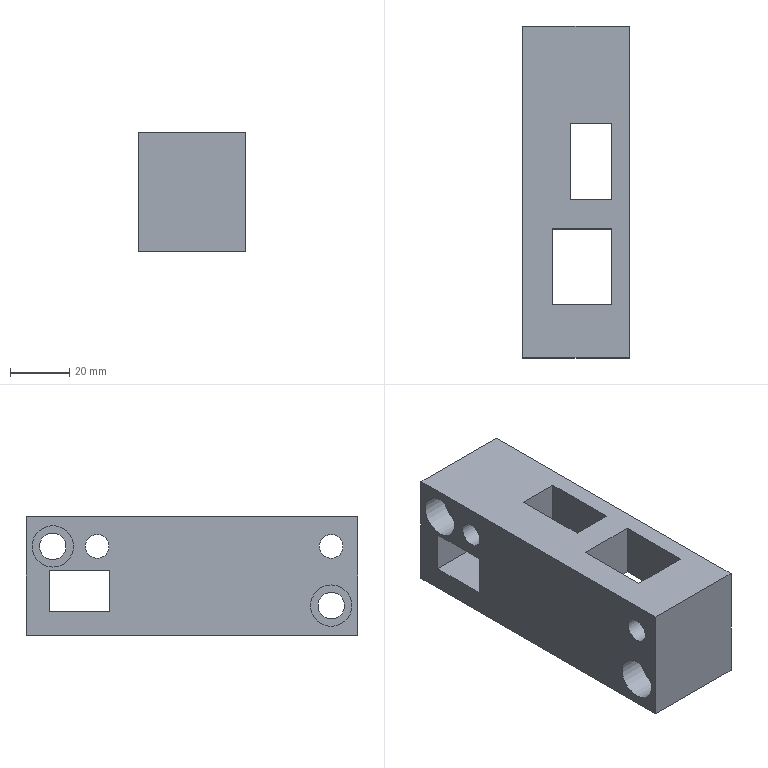Part | STEP file | solid 88 | 1 solid | 34 faces | box 36 x 112 x 40 mm | volume 94873 mm3 | plane 26 | cylinder 8 | commonest cylinder face diameters 8 x2 9 x2 10 x2 14 x2